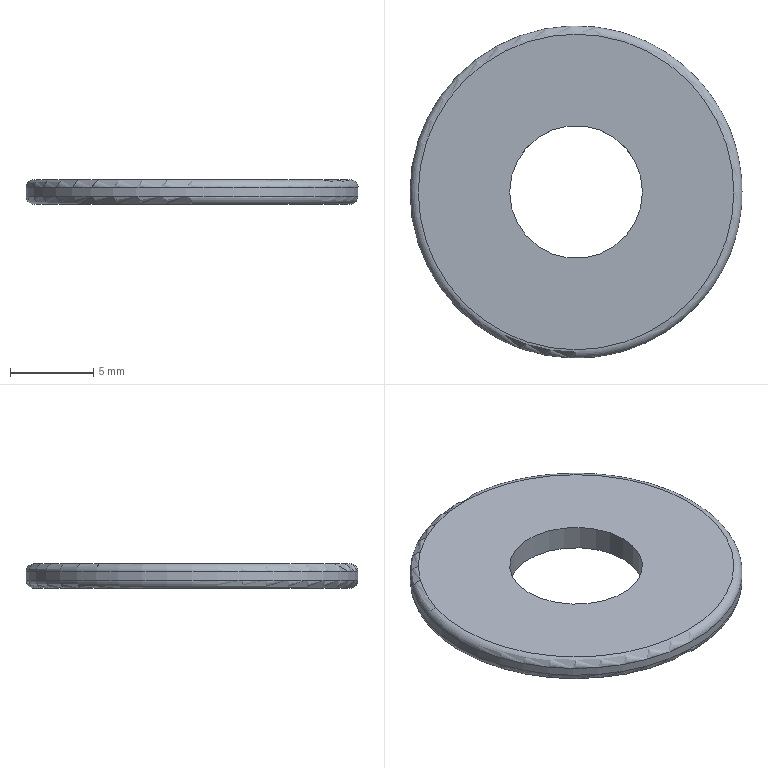Part | STEP file | Tube necking machine_id390_x_t | 1 solid | 6 faces | box 20 x 20 x 1.5 mm | volume 389.174 mm3 | cylinder 2 | plane 2 | torus 2 | commonest cylinder face diameters 8 x1 20 x1
STEP:
#1=CARTESIAN_POINT('',(0.,0.,0.));
#2=DIRECTION('',(0.,0.,1.));
#3=DIRECTION('',(1.,0.,0.));
#4=AXIS2_PLACEMENT_3D('',#1,#2,#3);
#5=CARTESIAN_POINT('',(-179.5,28.,199.5));
#6=VERTEX_POINT('',#5);
#7=CARTESIAN_POINT('',(-169.5,28.,199.5));
#8=DIRECTION('',(0.,0.,-1.));
#9=DIRECTION('',(-1.,0.,0.));
#10=AXIS2_PLACEMENT_3D('',#7,#8,#9);
#11=CIRCLE('',#10,10.);
#12=CARTESIAN_POINT('',(-169.5,28.,198.5));
#13=DIRECTION('',(0.,0.,1.));
#14=DIRECTION('',(1.,0.,0.));
#15=AXIS2_PLACEMENT_3D('',#12,#13,#14);
#16=CYLINDRICAL_SURFACE('',#15,10.);
#17=CARTESIAN_POINT('',(9.425,1.));
#18=DIRECTION('',(-1.,0.));
#19=VECTOR('',#18,1.);
#20=LINE('',#17,#19);
#21=(GEOMETRIC_REPRESENTATION_CONTEXT(2)PARAMETRIC_REPRESENTATION_CONTEXT()REPRESENTATION_CONTEXT('',''));
#22=DEFINITIONAL_REPRESENTATION('',(#20),#21);
#23=PCURVE('',#16,#22);
#24=CARTESIAN_POINT('',(-169.5,28.,199.5));
#25=DIRECTION('',(0.,0.,-1.));
#26=DIRECTION('',(-1.,0.,0.));
#27=AXIS2_PLACEMENT_3D('',#24,#25,#26);
#28=TOROIDAL_SURFACE('',#27,9.5,0.5);
#29=CARTESIAN_POINT('',(0.,6.283));
#30=DIRECTION('',(1.,0.));
#31=VECTOR('',#30,1.);
#32=LINE('',#29,#31);
#33=(GEOMETRIC_REPRESENTATION_CONTEXT(2)PARAMETRIC_REPRESENTATION_CONTEXT()REPRESENTATION_CONTEXT('',''));
#34=DEFINITIONAL_REPRESENTATION('',(#32),#33);
#35=PCURVE('',#28,#34);
#36=SURFACE_CURVE('',#11,(#23,#35),.PCURVE_S1.);
#37=EDGE_CURVE('',#6,#6,#36,.T.);
#38=ORIENTED_EDGE('',*,*,#37,.T.);
#39=CARTESIAN_POINT('',(-179.5,28.,199.));
#40=VERTEX_POINT('',#39);
#41=CARTESIAN_POINT('',(-179.5,28.,199.));
#42=CARTESIAN_POINT('',(-179.5,28.,199.5));
#43=B_SPLINE_CURVE_WITH_KNOTS('',1,(#41,#42),.UNSPECIFIED.,.F.,.F.,(2,2),(0.5,1.),.PIECEWISE_BEZIER_KNOTS.);
#44=CARTESIAN_POINT('',(3.142,0.));
#45=DIRECTION('',(0.,1.));
#46=VECTOR('',#45,1.);
#47=LINE('',#44,#46);
#48=(GEOMETRIC_REPRESENTATION_CONTEXT(2)PARAMETRIC_REPRESENTATION_CONTEXT()REPRESENTATION_CONTEXT('',''));
#49=DEFINITIONAL_REPRESENTATION('',(#47),#48);
#50=PCURVE('',#16,#49);
#51=CARTESIAN_POINT('',(9.425,0.));
#52=DIRECTION('',(0.,1.));
#53=VECTOR('',#52,1.);
#54=LINE('',#51,#53);
#55=(GEOMETRIC_REPRESENTATION_CONTEXT(2)PARAMETRIC_REPRESENTATION_CONTEXT()REPRESENTATION_CONTEXT('',''));
#56=DEFINITIONAL_REPRESENTATION('',(#54),#55);
#57=PCURVE('',#16,#56);
#58=SEAM_CURVE('',#43,(#50,#57),.PCURVE_S1.);
#59=EDGE_CURVE('',#40,#6,#58,.T.);
#60=ORIENTED_EDGE('',*,*,#59,.F.);
#61=CARTESIAN_POINT('',(-169.5,28.,199.));
#62=DIRECTION('',(0.,0.,1.));
#63=DIRECTION('',(-1.,0.,0.));
#64=AXIS2_PLACEMENT_3D('',#61,#62,#63);
#65=CIRCLE('',#64,10.);
#66=CARTESIAN_POINT('',(3.142,0.5));
#67=DIRECTION('',(1.,0.));
#68=VECTOR('',#67,1.);
#69=LINE('',#66,#68);
#70=(GEOMETRIC_REPRESENTATION_CONTEXT(2)PARAMETRIC_REPRESENTATION_CONTEXT()REPRESENTATION_CONTEXT('',''));
#71=DEFINITIONAL_REPRESENTATION('',(#69),#70);
#72=PCURVE('',#16,#71);
#73=CARTESIAN_POINT('',(-169.5,28.,199.));
#74=DIRECTION('',(0.,0.,-1.));
#75=DIRECTION('',(-1.,0.,0.));
#76=AXIS2_PLACEMENT_3D('',#73,#74,#75);
#77=TOROIDAL_SURFACE('',#76,9.5,0.5);
#78=CARTESIAN_POINT('',(6.283,6.283));
#79=DIRECTION('',(-1.,0.));
#80=VECTOR('',#79,1.);
#81=LINE('',#78,#80);
#82=(GEOMETRIC_REPRESENTATION_CONTEXT(2)PARAMETRIC_REPRESENTATION_CONTEXT()REPRESENTATION_CONTEXT('',''));
#83=DEFINITIONAL_REPRESENTATION('',(#81),#82);
#84=PCURVE('',#77,#83);
#85=SURFACE_CURVE('',#65,(#72,#84),.PCURVE_S1.);
#86=EDGE_CURVE('',#40,#40,#85,.T.);
#87=ORIENTED_EDGE('',*,*,#86,.T.);
#88=ORIENTED_EDGE('',*,*,#59,.T.);
#89=EDGE_LOOP('',(#38,#60,#87,#88));
#90=FACE_BOUND('',#89,.T.);
#91=ADVANCED_FACE('',(#90),#16,.T.);
#92=CARTESIAN_POINT('',(-173.5,28.,198.5));
#93=VERTEX_POINT('',#92);
#94=CARTESIAN_POINT('',(-169.5,28.,198.5));
#95=DIRECTION('',(0.,0.,1.));
#96=DIRECTION('',(-1.,0.,0.));
#97=AXIS2_PLACEMENT_3D('',#94,#95,#96);
#98=CIRCLE('',#97,4.);
#99=CARTESIAN_POINT('',(-169.5,28.,198.5));
#100=DIRECTION('',(0.,0.,-1.));
#101=DIRECTION('',(-1.,0.,0.));
#102=AXIS2_PLACEMENT_3D('',#99,#100,#101);
#103=PLANE('',#102);
#104=CARTESIAN_POINT('',(4.,0.));
#105=CARTESIAN_POINT('',(4.,-6.928));
#106=CARTESIAN_POINT('',(-2.,-3.464));
#107=CARTESIAN_POINT('',(-8.,0.));
#108=CARTESIAN_POINT('',(-2.,3.464));
#109=CARTESIAN_POINT('',(4.,6.928));
#110=CARTESIAN_POINT('',(4.,0.));
#111=(BOUNDED_CURVE()B_SPLINE_CURVE(2,(#104,#105,#106,#107,#108,#109,#110),.UNSPECIFIED.,.T.,.F.)B_SPLINE_CURVE_WITH_KNOTS((1,2,2,2,2,1),(-2.094,0.,2.094,4.189,6.283,8.378),.UNSPECIFIED.)CURVE()GEOMETRIC_REPRESENTATION_ITEM()RATIONAL_B_SPLINE_CURVE((1.,0.5,1.,0.5,1.,0.5,1.))REPRESENTATION_ITEM(''));
#112=(GEOMETRIC_REPRESENTATION_CONTEXT(2)PARAMETRIC_REPRESENTATION_CONTEXT()REPRESENTATION_CONTEXT('',''));
#113=DEFINITIONAL_REPRESENTATION('',(#111),#112);
#114=PCURVE('',#103,#113);
#115=CARTESIAN_POINT('',(-169.5,28.,218.9));
#116=DIRECTION('',(0.,0.,-1.));
#117=DIRECTION('',(-1.,0.,0.));
#118=AXIS2_PLACEMENT_3D('',#115,#116,#117);
#119=CYLINDRICAL_SURFACE('',#118,4.);
#120=CARTESIAN_POINT('',(6.283,20.4));
#121=DIRECTION('',(-1.,0.));
#122=VECTOR('',#121,1.);
#123=LINE('',#120,#122);
#124=(GEOMETRIC_REPRESENTATION_CONTEXT(2)PARAMETRIC_REPRESENTATION_CONTEXT()REPRESENTATION_CONTEXT('',''));
#125=DEFINITIONAL_REPRESENTATION('',(#123),#124);
#126=PCURVE('',#119,#125);
#127=SURFACE_CURVE('',#98,(#114,#126),.PCURVE_S1.);
#128=EDGE_CURVE('',#93,#93,#127,.T.);
#129=ORIENTED_EDGE('',*,*,#128,.T.);
#130=EDGE_LOOP('',(#129));
#131=FACE_BOUND('',#130,.T.);
#132=CARTESIAN_POINT('',(-179.,28.,198.5));
#133=VERTEX_POINT('',#132);
#134=CARTESIAN_POINT('',(-169.5,28.,198.5));
#135=DIRECTION('',(0.,0.,-1.));
#136=DIRECTION('',(-1.,0.,0.));
#137=AXIS2_PLACEMENT_3D('',#134,#135,#136);
#138=CIRCLE('',#137,9.5);
#139=CARTESIAN_POINT('',(0.,0.));
#140=DIRECTION('',(1.,0.));
#141=AXIS2_PLACEMENT_2D('',#139,#140);
#142=CIRCLE('',#141,9.5);
#143=(GEOMETRIC_REPRESENTATION_CONTEXT(2)PARAMETRIC_REPRESENTATION_CONTEXT()REPRESENTATION_CONTEXT('',''));
#144=DEFINITIONAL_REPRESENTATION('',(#142),#143);
#145=PCURVE('',#103,#144);
#146=CARTESIAN_POINT('',(0.,7.854));
#147=DIRECTION('',(1.,0.));
#148=VECTOR('',#147,1.);
#149=LINE('',#146,#148);
#150=(GEOMETRIC_REPRESENTATION_CONTEXT(2)PARAMETRIC_REPRESENTATION_CONTEXT()REPRESENTATION_CONTEXT('',''));
#151=DEFINITIONAL_REPRESENTATION('',(#149),#150);
#152=PCURVE('',#77,#151);
#153=SURFACE_CURVE('',#138,(#145,#152),.PCURVE_S1.);
#154=EDGE_CURVE('',#133,#133,#153,.T.);
#155=ORIENTED_EDGE('',*,*,#154,.T.);
#156=EDGE_LOOP('',(#155));
#157=FACE_BOUND('',#156,.T.);
#158=ADVANCED_FACE('',(#131,#157),#103,.T.);
#159=CARTESIAN_POINT('',(-173.5,28.,200.));
#160=VERTEX_POINT('',#159);
#161=CARTESIAN_POINT('',(-169.5,28.,200.));
#162=DIRECTION('',(0.,0.,1.));
#163=DIRECTION('',(-1.,0.,0.));
#164=AXIS2_PLACEMENT_3D('',#161,#162,#163);
#165=CIRCLE('',#164,4.);
#166=CARTESIAN_POINT('',(-169.5,28.,200.));
#167=DIRECTION('',(0.,0.,-1.));
#168=DIRECTION('',(-1.,0.,0.));
#169=AXIS2_PLACEMENT_3D('',#166,#167,#168);
#170=PLANE('',#169);
#171=CARTESIAN_POINT('',(4.,0.));
#172=CARTESIAN_POINT('',(4.,-6.928));
#173=CARTESIAN_POINT('',(-2.,-3.464));
#174=CARTESIAN_POINT('',(-8.,0.));
#175=CARTESIAN_POINT('',(-2.,3.464));
#176=CARTESIAN_POINT('',(4.,6.928));
#177=CARTESIAN_POINT('',(4.,0.));
#178=(BOUNDED_CURVE()B_SPLINE_CURVE(2,(#171,#172,#173,#174,#175,#176,#177),.UNSPECIFIED.,.T.,.F.)B_SPLINE_CURVE_WITH_KNOTS((1,2,2,2,2,1),(-2.094,0.,2.094,4.189,6.283,8.378),.UNSPECIFIED.)CURVE()GEOMETRIC_REPRESENTATION_ITEM()RATIONAL_B_SPLINE_CURVE((1.,0.5,1.,0.5,1.,0.5,1.))REPRESENTATION_ITEM(''));
#179=(GEOMETRIC_REPRESENTATION_CONTEXT(2)PARAMETRIC_REPRESENTATION_CONTEXT()REPRESENTATION_CONTEXT('',''));
#180=DEFINITIONAL_REPRESENTATION('',(#178),#179);
#181=PCURVE('',#170,#180);
#182=CARTESIAN_POINT('',(6.283,18.9));
#183=DIRECTION('',(-1.,0.));
#184=VECTOR('',#183,1.);
#185=LINE('',#182,#184);
#186=(GEOMETRIC_REPRESENTATION_CONTEXT(2)PARAMETRIC_REPRESENTATION_CONTEXT()REPRESENTATION_CONTEXT('',''));
#187=DEFINITIONAL_REPRESENTATION('',(#185),#186);
#188=PCURVE('',#119,#187);
#189=SURFACE_CURVE('',#165,(#181,#188),.PCURVE_S1.);
#190=EDGE_CURVE('',#160,#160,#189,.T.);
#191=ORIENTED_EDGE('',*,*,#190,.F.);
#192=EDGE_LOOP('',(#191));
#193=FACE_BOUND('',#192,.T.);
#194=CARTESIAN_POINT('',(-179.,28.,200.));
#195=VERTEX_POINT('',#194);
#196=CARTESIAN_POINT('',(-169.5,28.,200.));
#197=DIRECTION('',(0.,0.,1.));
#198=DIRECTION('',(-1.,0.,0.));
#199=AXIS2_PLACEMENT_3D('',#196,#197,#198);
#200=CIRCLE('',#199,9.5);
#201=CARTESIAN_POINT('',(9.5,0.));
#202=CARTESIAN_POINT('',(9.5,-16.454));
#203=CARTESIAN_POINT('',(-4.75,-8.227));
#204=CARTESIAN_POINT('',(-19.,0.));
#205=CARTESIAN_POINT('',(-4.75,8.227));
#206=CARTESIAN_POINT('',(9.5,16.454));
#207=CARTESIAN_POINT('',(9.5,0.));
#208=(BOUNDED_CURVE()B_SPLINE_CURVE(2,(#201,#202,#203,#204,#205,#206,#207),.UNSPECIFIED.,.T.,.F.)B_SPLINE_CURVE_WITH_KNOTS((1,2,2,2,2,1),(-2.094,0.,2.094,4.189,6.283,8.378),.UNSPECIFIED.)CURVE()GEOMETRIC_REPRESENTATION_ITEM()RATIONAL_B_SPLINE_CURVE((1.,0.5,1.,0.5,1.,0.5,1.))REPRESENTATION_ITEM(''));
#209=(GEOMETRIC_REPRESENTATION_CONTEXT(2)PARAMETRIC_REPRESENTATION_CONTEXT()REPRESENTATION_CONTEXT('',''));
#210=DEFINITIONAL_REPRESENTATION('',(#208),#209);
#211=PCURVE('',#170,#210);
#212=CARTESIAN_POINT('',(6.283,4.712));
#213=DIRECTION('',(-1.,0.));
#214=VECTOR('',#213,1.);
#215=LINE('',#212,#214);
#216=(GEOMETRIC_REPRESENTATION_CONTEXT(2)PARAMETRIC_REPRESENTATION_CONTEXT()REPRESENTATION_CONTEXT('',''));
#217=DEFINITIONAL_REPRESENTATION('',(#215),#216);
#218=PCURVE('',#28,#217);
#219=SURFACE_CURVE('',#200,(#211,#218),.PCURVE_S1.);
#220=EDGE_CURVE('',#195,#195,#219,.T.);
#221=ORIENTED_EDGE('',*,*,#220,.T.);
#222=EDGE_LOOP('',(#221));
#223=FACE_BOUND('',#222,.T.);
#224=ADVANCED_FACE('',(#193,#223),#170,.F.);
#225=ORIENTED_EDGE('',*,*,#220,.F.);
#226=CARTESIAN_POINT('',(-179.,28.,200.));
#227=CARTESIAN_POINT('',(-179.134,28.,200.));
#228=CARTESIAN_POINT('',(-179.264,28.,199.957));
#229=CARTESIAN_POINT('',(-179.376,28.,199.876));
#230=CARTESIAN_POINT('',(-179.457,28.,199.764));
#231=CARTESIAN_POINT('',(-179.5,28.,199.634));
#232=CARTESIAN_POINT('',(-179.5,28.,199.5));
#233=(BOUNDED_CURVE()B_SPLINE_CURVE(6,(#226,#227,#228,#229,#230,#231,#232),.UNSPECIFIED.,.F.,.F.)B_SPLINE_CURVE_WITH_KNOTS((7,7),(4.712,6.283),.PIECEWISE_BEZIER_KNOTS.)CURVE()GEOMETRIC_REPRESENTATION_ITEM()RATIONAL_B_SPLINE_CURVE((1.031,1.01,0.9979,0.994,0.9979,1.01,1.031))REPRESENTATION_ITEM(''));
#234=CARTESIAN_POINT('',(6.283,0.));
#235=DIRECTION('',(0.,1.));
#236=VECTOR('',#235,1.);
#237=LINE('',#234,#236);
#238=(GEOMETRIC_REPRESENTATION_CONTEXT(2)PARAMETRIC_REPRESENTATION_CONTEXT()REPRESENTATION_CONTEXT('',''));
#239=DEFINITIONAL_REPRESENTATION('',(#237),#238);
#240=PCURVE('',#28,#239);
#241=CARTESIAN_POINT('',(0.,0.));
#242=DIRECTION('',(0.,1.));
#243=VECTOR('',#242,1.);
#244=LINE('',#241,#243);
#245=(GEOMETRIC_REPRESENTATION_CONTEXT(2)PARAMETRIC_REPRESENTATION_CONTEXT()REPRESENTATION_CONTEXT('',''));
#246=DEFINITIONAL_REPRESENTATION('',(#244),#245);
#247=PCURVE('',#28,#246);
#248=SEAM_CURVE('',#233,(#240,#247),.PCURVE_S1.);
#249=EDGE_CURVE('',#195,#6,#248,.T.);
#250=ORIENTED_EDGE('',*,*,#249,.T.);
#251=ORIENTED_EDGE('',*,*,#37,.F.);
#252=ORIENTED_EDGE('',*,*,#249,.F.);
#253=EDGE_LOOP('',(#225,#250,#251,#252));
#254=FACE_BOUND('',#253,.T.);
#255=ADVANCED_FACE('',(#254),#28,.T.);
#256=ORIENTED_EDGE('',*,*,#86,.F.);
#257=CARTESIAN_POINT('',(-179.5,28.,199.));
#258=CARTESIAN_POINT('',(-179.5,28.,198.866));
#259=CARTESIAN_POINT('',(-179.457,28.,198.736));
#260=CARTESIAN_POINT('',(-179.376,28.,198.624));
#261=CARTESIAN_POINT('',(-179.264,28.,198.543));
#262=CARTESIAN_POINT('',(-179.134,28.,198.5));
#263=CARTESIAN_POINT('',(-179.,28.,198.5));
#264=(BOUNDED_CURVE()B_SPLINE_CURVE(6,(#257,#258,#259,#260,#261,#262,#263),.UNSPECIFIED.,.F.,.F.)B_SPLINE_CURVE_WITH_KNOTS((7,7),(0.,1.571),.PIECEWISE_BEZIER_KNOTS.)CURVE()GEOMETRIC_REPRESENTATION_ITEM()RATIONAL_B_SPLINE_CURVE((1.031,1.01,0.9979,0.994,0.9979,1.01,1.031))REPRESENTATION_ITEM(''));
#265=CARTESIAN_POINT('',(6.283,6.283));
#266=DIRECTION('',(0.,1.));
#267=VECTOR('',#266,1.);
#268=LINE('',#265,#267);
#269=(GEOMETRIC_REPRESENTATION_CONTEXT(2)PARAMETRIC_REPRESENTATION_CONTEXT()REPRESENTATION_CONTEXT('',''));
#270=DEFINITIONAL_REPRESENTATION('',(#268),#269);
#271=PCURVE('',#77,#270);
#272=CARTESIAN_POINT('',(0.,6.283));
#273=DIRECTION('',(0.,1.));
#274=VECTOR('',#273,1.);
#275=LINE('',#272,#274);
#276=(GEOMETRIC_REPRESENTATION_CONTEXT(2)PARAMETRIC_REPRESENTATION_CONTEXT()REPRESENTATION_CONTEXT('',''));
#277=DEFINITIONAL_REPRESENTATION('',(#275),#276);
#278=PCURVE('',#77,#277);
#279=SEAM_CURVE('',#264,(#271,#278),.PCURVE_S1.);
#280=EDGE_CURVE('',#40,#133,#279,.T.);
#281=ORIENTED_EDGE('',*,*,#280,.T.);
#282=ORIENTED_EDGE('',*,*,#154,.F.);
#283=ORIENTED_EDGE('',*,*,#280,.F.);
#284=EDGE_LOOP('',(#256,#281,#282,#283));
#285=FACE_BOUND('',#284,.T.);
#286=ADVANCED_FACE('',(#285),#77,.T.);
#287=ORIENTED_EDGE('',*,*,#128,.T.);
#288=CARTESIAN_POINT('',(-173.5,28.,200.));
#289=CARTESIAN_POINT('',(-173.5,28.,198.5));
#290=B_SPLINE_CURVE_WITH_KNOTS('',1,(#288,#289),.UNSPECIFIED.,.F.,.F.,(2,2),(18.9,20.4),.PIECEWISE_BEZIER_KNOTS.);
#291=CARTESIAN_POINT('',(0.,0.));
#292=DIRECTION('',(0.,1.));
#293=VECTOR('',#292,1.);
#294=LINE('',#291,#293);
#295=(GEOMETRIC_REPRESENTATION_CONTEXT(2)PARAMETRIC_REPRESENTATION_CONTEXT()REPRESENTATION_CONTEXT('',''));
#296=DEFINITIONAL_REPRESENTATION('',(#294),#295);
#297=PCURVE('',#119,#296);
#298=CARTESIAN_POINT('',(6.283,0.));
#299=DIRECTION('',(0.,1.));
#300=VECTOR('',#299,1.);
#301=LINE('',#298,#300);
#302=(GEOMETRIC_REPRESENTATION_CONTEXT(2)PARAMETRIC_REPRESENTATION_CONTEXT()REPRESENTATION_CONTEXT('',''));
#303=DEFINITIONAL_REPRESENTATION('',(#301),#302);
#304=PCURVE('',#119,#303);
#305=SEAM_CURVE('',#290,(#297,#304),.PCURVE_S1.);
#306=EDGE_CURVE('',#160,#93,#305,.T.);
#307=ORIENTED_EDGE('',*,*,#306,.F.);
#308=ORIENTED_EDGE('',*,*,#190,.F.);
#309=ORIENTED_EDGE('',*,*,#306,.T.);
#310=EDGE_LOOP('',(#287,#307,#308,#309));
#311=FACE_BOUND('',#310,.F.);
#312=ADVANCED_FACE('',(#311),#119,.F.);
#313=CLOSED_SHELL('',(#91,#158,#224,#255,#286,#312));
#314=MANIFOLD_SOLID_BREP('',#313);
#315=(LENGTH_UNIT()NAMED_UNIT(*)SI_UNIT(.MILLI.,.METRE.));
#316=UNCERTAINTY_MEASURE_WITH_UNIT(LENGTH_MEASURE(0.00001),#315,'','');
#317=(NAMED_UNIT(*)PLANE_ANGLE_UNIT()SI_UNIT($,.RADIAN.));
#318=(NAMED_UNIT(*)SI_UNIT($,.STERADIAN.)SOLID_ANGLE_UNIT());
#319=(GEOMETRIC_REPRESENTATION_CONTEXT(3)GLOBAL_UNCERTAINTY_ASSIGNED_CONTEXT((#316))GLOBAL_UNIT_ASSIGNED_CONTEXT((#315,#317,#318))REPRESENTATION_CONTEXT('',''));
#320=ADVANCED_BREP_SHAPE_REPRESENTATION('',(#4,#314),#319);